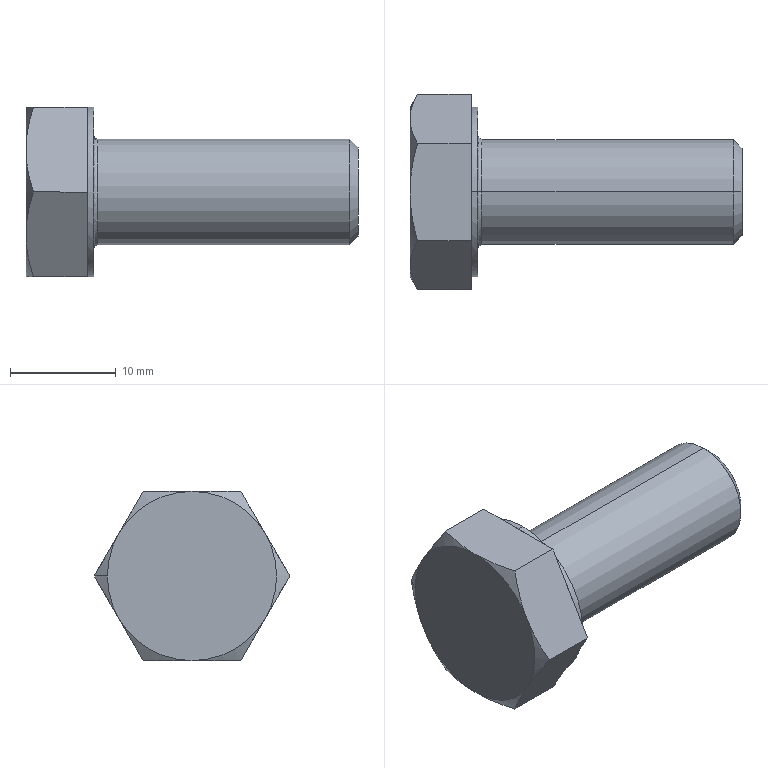Part | STEP file | Microwave Drying Flat Conveyor-hex screw gradeab_din_DIN EN 24017 - M10 x 25-N_Default | 1 solid | 30 faces | box 31.4 x 18.475 x 16 mm | volume 3356 mm3 | plane 15 | cone 9 | cylinder 4 | spline 2 | commonest cylinder face diameters 10 x2 16 x2
STEP:
#1=CARTESIAN_POINT('',(6.4,0.,5.4));
#2=VERTEX_POINT('',#1);
#3=CARTESIAN_POINT('',(6.4,0.,-5.4));
#4=VERTEX_POINT('',#3);
#5=CARTESIAN_POINT('',(6.4,0.,5.4));
#6=CARTESIAN_POINT('',(6.4,0.1651,5.4));
#7=CARTESIAN_POINT('',(6.4,0.4117,5.389));
#8=CARTESIAN_POINT('',(6.4,0.6977,5.356));
#9=CARTESIAN_POINT('',(6.4,0.8403,5.334));
#10=CARTESIAN_POINT('',(6.4,0.9013,5.324));
#11=CARTESIAN_POINT('',(6.4,0.942,5.317));
#12=CARTESIAN_POINT('',(6.4,0.9611,5.314));
#13=CARTESIAN_POINT('',(6.4,1.155,5.278));
#14=CARTESIAN_POINT('',(6.4,1.409,5.218));
#15=CARTESIAN_POINT('',(6.4,1.7,5.127));
#16=CARTESIAN_POINT('',(6.4,1.824,5.083));
#17=CARTESIAN_POINT('',(6.4,1.906,5.053));
#18=CARTESIAN_POINT('',(6.4,1.945,5.038));
#19=CARTESIAN_POINT('',(6.4,2.157,4.954));
#20=CARTESIAN_POINT('',(6.4,2.405,4.841));
#21=CARTESIAN_POINT('',(6.4,2.644,4.709));
#22=CARTESIAN_POINT('',(6.4,2.801,4.618));
#23=CARTESIAN_POINT('',(6.4,2.877,4.571));
#24=CARTESIAN_POINT('',(6.4,3.267,4.316));
#25=CARTESIAN_POINT('',(6.4,3.555,4.082));
#26=CARTESIAN_POINT('',(6.4,3.95,3.687));
#27=CARTESIAN_POINT('',(6.4,4.137,3.48));
#28=CARTESIAN_POINT('',(6.4,4.306,3.26));
#29=CARTESIAN_POINT('',(6.4,4.416,3.11));
#30=CARTESIAN_POINT('',(6.4,4.47,3.031));
#31=CARTESIAN_POINT('',(6.4,4.62,2.802));
#32=CARTESIAN_POINT('',(6.4,4.757,2.567));
#33=CARTESIAN_POINT('',(6.4,4.896,2.281));
#34=CARTESIAN_POINT('',(6.4,4.951,2.156));
#35=CARTESIAN_POINT('',(6.4,4.987,2.072));
#36=CARTESIAN_POINT('',(6.4,5.005,2.028));
#37=CARTESIAN_POINT('',(6.4,5.085,1.825));
#38=CARTESIAN_POINT('',(6.4,5.17,1.577));
#39=CARTESIAN_POINT('',(6.4,5.247,1.282));
#40=CARTESIAN_POINT('',(6.4,5.28,1.133));
#41=CARTESIAN_POINT('',(6.4,5.293,1.069));
#42=CARTESIAN_POINT('',(6.4,5.302,1.026));
#43=CARTESIAN_POINT('',(6.4,5.306,1.003));
#44=CARTESIAN_POINT('',(6.4,5.37,0.6582));
#45=CARTESIAN_POINT('',(6.4,5.4,0.3299));
#46=CARTESIAN_POINT('',(6.4,5.4,-0.165));
#47=CARTESIAN_POINT('',(6.4,5.389,-0.4115));
#48=CARTESIAN_POINT('',(6.4,5.356,-0.6976));
#49=CARTESIAN_POINT('',(6.4,5.335,-0.8402));
#50=CARTESIAN_POINT('',(6.4,5.324,-0.9013));
#51=CARTESIAN_POINT('',(6.4,5.317,-0.9419));
#52=CARTESIAN_POINT('',(6.4,5.314,-0.9611));
#53=CARTESIAN_POINT('',(6.4,5.278,-1.155));
#54=CARTESIAN_POINT('',(6.4,5.218,-1.409));
#55=CARTESIAN_POINT('',(6.4,5.127,-1.7));
#56=CARTESIAN_POINT('',(6.4,5.083,-1.824));
#57=CARTESIAN_POINT('',(6.4,5.053,-1.906));
#58=CARTESIAN_POINT('',(6.4,5.038,-1.945));
#59=CARTESIAN_POINT('',(6.4,4.954,-2.157));
#60=CARTESIAN_POINT('',(6.4,4.841,-2.405));
#61=CARTESIAN_POINT('',(6.4,4.709,-2.644));
#62=CARTESIAN_POINT('',(6.4,4.618,-2.801));
#63=CARTESIAN_POINT('',(6.4,4.571,-2.877));
#64=CARTESIAN_POINT('',(6.4,4.316,-3.267));
#65=CARTESIAN_POINT('',(6.4,4.082,-3.555));
#66=CARTESIAN_POINT('',(6.4,3.687,-3.95));
#67=CARTESIAN_POINT('',(6.4,3.48,-4.137));
#68=CARTESIAN_POINT('',(6.4,3.26,-4.306));
#69=CARTESIAN_POINT('',(6.4,3.11,-4.416));
#70=CARTESIAN_POINT('',(6.4,3.031,-4.47));
#71=CARTESIAN_POINT('',(6.4,2.802,-4.62));
#72=CARTESIAN_POINT('',(6.4,2.567,-4.757));
#73=CARTESIAN_POINT('',(6.4,2.281,-4.896));
#74=CARTESIAN_POINT('',(6.4,2.156,-4.951));
#75=CARTESIAN_POINT('',(6.4,2.072,-4.987));
#76=CARTESIAN_POINT('',(6.4,2.028,-5.005));
#77=CARTESIAN_POINT('',(6.4,1.825,-5.085));
#78=CARTESIAN_POINT('',(6.4,1.577,-5.17));
#79=CARTESIAN_POINT('',(6.4,1.282,-5.247));
#80=CARTESIAN_POINT('',(6.4,1.133,-5.28));
#81=CARTESIAN_POINT('',(6.4,1.069,-5.293));
#82=CARTESIAN_POINT('',(6.4,1.026,-5.302));
#83=CARTESIAN_POINT('',(6.4,1.003,-5.306));
#84=CARTESIAN_POINT('',(6.4,0.658,-5.37));
#85=CARTESIAN_POINT('',(6.4,0.3305,-5.4));
#86=CARTESIAN_POINT('',(6.4,0.,-5.4));
#87=B_SPLINE_CURVE_WITH_KNOTS('',3,(#5,#6,#7,#8,#9,#10,#11,#12,#13,#14,#15,#16,#17,#18,#19,#20,#21,#22,#23,#24,#25,#26,#27,#28,#29,#30,#31,#32,#33,#34,#35,#36,#37,#38,#39,#40,#41,#42,#43,#44,#45,#46,#47,#48,#49,#50,#51,#52,#53,#54,#55,#56,#57,#58,#59,#60,#61,#62,#63,#64,#65,#66,#67,#68,#69,#70,#71,#72,#73,#74,#75,#76,#77,#78,#79,#80,#81,#82,#83,#84,#85,#86),.UNSPECIFIED.,.F.,.F.,(4,1,1,1,2,2,1,1,2,2,1,2,2,2,1,2,2,1,1,2,2,1,1,1,2,2,2,1,1,1,2,2,1,1,2,2,1,2,2,2,1,2,2,1,1,2,2,1,1,1,2,2,4),(0.,0.03125,0.04687,0.05469,0.05859,0.0625,0.09375,0.1094,0.1172,0.125,0.1562,0.1719,0.1875,0.25,0.2812,0.2969,0.3125,0.3437,0.3594,0.3672,0.375,0.4062,0.4219,0.4297,0.4336,0.4375,0.5,0.5312,0.5469,0.5547,0.5586,0.5625,0.5937,0.6094,0.6172,0.625,0.6562,0.6719,0.6875,0.75,0.7812,0.7969,0.8125,0.8437,0.8594,0.8672,0.875,0.9062,0.9219,0.9297,0.9336,0.9375,1.),.UNSPECIFIED.);
#88=EDGE_CURVE('',#2,#4,#87,.T.);
#89=ORIENTED_EDGE('',*,*,#88,.F.);
#90=CARTESIAN_POINT('',(6.8,0.,5.));
#91=VERTEX_POINT('',#90);
#92=CARTESIAN_POINT('',(6.8,0.,5.4));
#93=DIRECTION('',(0.,-1.,0.));
#94=DIRECTION('',(0.,0.,1.));
#95=AXIS2_PLACEMENT_3D('',#92,#93,#94);
#96=CIRCLE('',#95,0.4);
#97=EDGE_CURVE('',#2,#91,#96,.T.);
#98=ORIENTED_EDGE('',*,*,#97,.T.);
#99=CARTESIAN_POINT('',(6.8,0.,-5.));
#100=VERTEX_POINT('',#99);
#101=CARTESIAN_POINT('',(6.8,0.,0.));
#102=DIRECTION('',(1.,0.,0.));
#103=DIRECTION('',(0.,0.,1.));
#104=AXIS2_PLACEMENT_3D('',#101,#102,#103);
#105=CIRCLE('',#104,5.);
#106=EDGE_CURVE('',#100,#91,#105,.T.);
#107=ORIENTED_EDGE('',*,*,#106,.F.);
#108=CARTESIAN_POINT('',(6.8,0.,-5.4));
#109=DIRECTION('',(0.,1.,0.));
#110=DIRECTION('',(0.,0.,-1.));
#111=AXIS2_PLACEMENT_3D('',#108,#109,#110);
#112=CIRCLE('',#111,0.4);
#113=EDGE_CURVE('',#4,#100,#112,.T.);
#114=ORIENTED_EDGE('',*,*,#113,.F.);
#115=EDGE_LOOP('',(#89,#98,#107,#114));
#116=FACE_OUTER_BOUND('',#115,.T.);
#117=CARTESIAN_POINT('',(6.4,0.,-5.4));
#118=CARTESIAN_POINT('',(6.4,10.8,-5.4));
#119=CARTESIAN_POINT('',(6.4,10.8,5.4));
#120=CARTESIAN_POINT('',(6.4,0.,5.4));
#121=CARTESIAN_POINT('',(6.4,0.,-5.166));
#122=CARTESIAN_POINT('',(6.4,10.331,-5.166));
#123=CARTESIAN_POINT('',(6.4,10.331,5.166));
#124=CARTESIAN_POINT('',(6.4,0.,5.166));
#125=CARTESIAN_POINT('',(6.566,0.,-5.));
#126=CARTESIAN_POINT('',(6.566,10.,-5.));
#127=CARTESIAN_POINT('',(6.566,10.,5.));
#128=CARTESIAN_POINT('',(6.566,0.,5.));
#129=CARTESIAN_POINT('',(6.8,0.,-5.));
#130=CARTESIAN_POINT('',(6.8,10.,-5.));
#131=CARTESIAN_POINT('',(6.8,10.,5.));
#132=CARTESIAN_POINT('',(6.8,0.,5.));
#133=(BOUNDED_SURFACE()B_SPLINE_SURFACE(3,3,((#117,#118,#119,#120),(#121,#122,#123,#124),(#125,#126,#127,#128),(#129,#130,#131,#132)),.UNSPECIFIED.,.F.,.F.,.F.)B_SPLINE_SURFACE_WITH_KNOTS((4,4),(4,4),(0.,1.),(0.,1.),.UNSPECIFIED.)GEOMETRIC_REPRESENTATION_ITEM()RATIONAL_B_SPLINE_SURFACE(((1.,0.3333,0.3333,1.),(0.8047,0.2682,0.2682,0.8047),(0.8047,0.2682,0.2682,0.8047),(1.,0.3333,0.3333,1.)))REPRESENTATION_ITEM('')SURFACE());
#134=ADVANCED_FACE('',(#116),#133,.F.);
#135=CARTESIAN_POINT('',(30.572,0.,5.));
#136=VERTEX_POINT('',#135);
#137=CARTESIAN_POINT('',(30.572,0.,-5.));
#138=VERTEX_POINT('',#137);
#139=CARTESIAN_POINT('',(30.572,0.,0.));
#140=DIRECTION('',(-1.,0.,0.));
#141=DIRECTION('',(0.,0.,1.));
#142=AXIS2_PLACEMENT_3D('',#139,#140,#141);
#143=CIRCLE('',#142,5.);
#144=EDGE_CURVE('',#136,#138,#143,.T.);
#145=ORIENTED_EDGE('',*,*,#144,.T.);
#146=CARTESIAN_POINT('',(0.,0.,-5.));
#147=DIRECTION('',(-1.,0.,0.));
#148=VECTOR('',#147,1000.);
#149=LINE('',#146,#148);
#150=EDGE_CURVE('',#138,#100,#149,.T.);
#151=ORIENTED_EDGE('',*,*,#150,.T.);
#152=ORIENTED_EDGE('',*,*,#106,.T.);
#153=CARTESIAN_POINT('',(0.,0.,5.));
#154=DIRECTION('',(-1.,0.,0.));
#155=VECTOR('',#154,1000.);
#156=LINE('',#153,#155);
#157=EDGE_CURVE('',#136,#91,#156,.T.);
#158=ORIENTED_EDGE('',*,*,#157,.F.);
#159=EDGE_LOOP('',(#145,#151,#152,#158));
#160=FACE_OUTER_BOUND('',#159,.T.);
#161=CARTESIAN_POINT('',(0.,0.,0.));
#162=DIRECTION('',(-1.,0.,0.));
#163=DIRECTION('',(0.,0.,1.));
#164=AXIS2_PLACEMENT_3D('',#161,#162,#163);
#165=CYLINDRICAL_SURFACE('',#164,5.);
#166=ADVANCED_FACE('',(#160),#165,.T.);
#167=CARTESIAN_POINT('',(31.4,0.,4.172));
#168=VERTEX_POINT('',#167);
#169=CARTESIAN_POINT('',(31.4,0.,-4.172));
#170=VERTEX_POINT('',#169);
#171=CARTESIAN_POINT('',(31.4,0.,0.));
#172=DIRECTION('',(-1.,0.,0.));
#173=DIRECTION('',(0.,0.,1.));
#174=AXIS2_PLACEMENT_3D('',#171,#172,#173);
#175=CIRCLE('',#174,4.172);
#176=EDGE_CURVE('',#168,#170,#175,.T.);
#177=ORIENTED_EDGE('',*,*,#176,.T.);
#178=CARTESIAN_POINT('',(30.572,0.,-5.));
#179=DIRECTION('',(-0.7071,0.,-0.7071));
#180=VECTOR('',#179,1000.);
#181=LINE('',#178,#180);
#182=EDGE_CURVE('',#170,#138,#181,.T.);
#183=ORIENTED_EDGE('',*,*,#182,.T.);
#184=ORIENTED_EDGE('',*,*,#144,.F.);
#185=CARTESIAN_POINT('',(30.572,0.,5.));
#186=DIRECTION('',(-0.7071,0.,0.7071));
#187=VECTOR('',#186,1000.);
#188=LINE('',#185,#187);
#189=EDGE_CURVE('',#168,#136,#188,.T.);
#190=ORIENTED_EDGE('',*,*,#189,.F.);
#191=EDGE_LOOP('',(#177,#183,#184,#190));
#192=FACE_OUTER_BOUND('',#191,.T.);
#193=CARTESIAN_POINT('',(30.572,0.,0.));
#194=DIRECTION('',(-1.,0.,0.));
#195=DIRECTION('',(0.,0.,1.));
#196=AXIS2_PLACEMENT_3D('',#193,#194,#195);
#197=CONICAL_SURFACE('',#196,5.,0.7854);
#198=ADVANCED_FACE('',(#192),#197,.T.);
#199=CARTESIAN_POINT('',(6.4,0.,-8.));
#200=VERTEX_POINT('',#199);
#201=CARTESIAN_POINT('',(6.4,0.,8.));
#202=VERTEX_POINT('',#201);
#203=CARTESIAN_POINT('',(6.4,0.,0.));
#204=DIRECTION('',(1.,0.,0.));
#205=DIRECTION('',(0.,0.,1.));
#206=AXIS2_PLACEMENT_3D('',#203,#204,#205);
#207=CIRCLE('',#206,8.);
#208=EDGE_CURVE('',#200,#202,#207,.T.);
#209=ORIENTED_EDGE('',*,*,#208,.F.);
#210=CARTESIAN_POINT('',(5.8,0.,-8.));
#211=VERTEX_POINT('',#210);
#212=CARTESIAN_POINT('',(0.,0.,-8.));
#213=DIRECTION('',(-1.,0.,0.));
#214=VECTOR('',#213,1000.);
#215=LINE('',#212,#214);
#216=EDGE_CURVE('',#200,#211,#215,.T.);
#217=ORIENTED_EDGE('',*,*,#216,.T.);
#218=CARTESIAN_POINT('',(5.8,6.928,-4.));
#219=VERTEX_POINT('',#218);
#220=CARTESIAN_POINT('',(5.8,0.,0.));
#221=DIRECTION('',(1.,0.,0.));
#222=DIRECTION('',(0.,0.,1.));
#223=AXIS2_PLACEMENT_3D('',#220,#221,#222);
#224=CIRCLE('',#223,8.);
#225=EDGE_CURVE('',#211,#219,#224,.T.);
#226=ORIENTED_EDGE('',*,*,#225,.T.);
#227=CARTESIAN_POINT('',(5.8,6.928,4.));
#228=VERTEX_POINT('',#227);
#229=CARTESIAN_POINT('',(5.8,0.,0.));
#230=DIRECTION('',(1.,0.,0.));
#231=DIRECTION('',(0.,0.,1.));
#232=AXIS2_PLACEMENT_3D('',#229,#230,#231);
#233=CIRCLE('',#232,8.);
#234=EDGE_CURVE('',#219,#228,#233,.T.);
#235=ORIENTED_EDGE('',*,*,#234,.T.);
#236=CARTESIAN_POINT('',(5.8,0.,8.));
#237=VERTEX_POINT('',#236);
#238=CARTESIAN_POINT('',(5.8,0.,0.));
#239=DIRECTION('',(1.,0.,0.));
#240=DIRECTION('',(0.,0.,1.));
#241=AXIS2_PLACEMENT_3D('',#238,#239,#240);
#242=CIRCLE('',#241,8.);
#243=EDGE_CURVE('',#228,#237,#242,.T.);
#244=ORIENTED_EDGE('',*,*,#243,.T.);
#245=CARTESIAN_POINT('',(0.,0.,8.));
#246=DIRECTION('',(-1.,0.,0.));
#247=VECTOR('',#246,1000.);
#248=LINE('',#245,#247);
#249=EDGE_CURVE('',#202,#237,#248,.T.);
#250=ORIENTED_EDGE('',*,*,#249,.F.);
#251=EDGE_LOOP('',(#209,#217,#226,#235,#244,#250));
#252=FACE_OUTER_BOUND('',#251,.T.);
#253=CARTESIAN_POINT('',(0.,0.,0.));
#254=DIRECTION('',(-1.,0.,0.));
#255=DIRECTION('',(0.,0.,1.));
#256=AXIS2_PLACEMENT_3D('',#253,#254,#255);
#257=CYLINDRICAL_SURFACE('',#256,8.);
#258=ADVANCED_FACE('',(#252),#257,.T.);
#259=CARTESIAN_POINT('',(0.,6.928,-4.));
#260=VERTEX_POINT('',#259);
#261=CARTESIAN_POINT('',(0.,8.,0.));
#262=VERTEX_POINT('',#261);
#263=CARTESIAN_POINT('',(0.,0.,0.));
#264=DIRECTION('',(1.,0.,0.));
#265=DIRECTION('',(0.,1.,0.));
#266=AXIS2_PLACEMENT_3D('',#263,#264,#265);
#267=CIRCLE('',#266,8.);
#268=EDGE_CURVE('',#260,#262,#267,.T.);
#269=ORIENTED_EDGE('',*,*,#268,.T.);
#270=CARTESIAN_POINT('',(0.7145,9.238,0.));
#271=VERTEX_POINT('',#270);
#272=CARTESIAN_POINT('',(0.7188,9.245,0.));
#273=DIRECTION('',(0.5,0.866,0.));
#274=VECTOR('',#273,1000.);
#275=LINE('',#272,#274);
#276=EDGE_CURVE('',#262,#271,#275,.T.);
#277=ORIENTED_EDGE('',*,*,#276,.T.);
#278=CARTESIAN_POINT('',(0.7145,9.238,0.));
#279=CARTESIAN_POINT('',(0.4967,8.86,-0.6534));
#280=CARTESIAN_POINT('',(0.3171,8.48,-1.312));
#281=CARTESIAN_POINT('',(0.06831,7.711,-2.644));
#282=CARTESIAN_POINT('',(0.,7.322,-3.317));
#283=CARTESIAN_POINT('',(0.,6.928,-4.));
#284=B_SPLINE_CURVE_WITH_KNOTS('',3,(#278,#279,#280,#281,#282,#283),.UNSPECIFIED.,.F.,.F.,(4,2,4),(0.,0.002337,0.004674),.UNSPECIFIED.);
#285=EDGE_CURVE('',#271,#260,#284,.T.);
#286=ORIENTED_EDGE('',*,*,#285,.T.);
#287=EDGE_LOOP('',(#269,#277,#286));
#288=FACE_OUTER_BOUND('',#287,.T.);
#289=CARTESIAN_POINT('',(0.7188,0.,0.));
#290=DIRECTION('',(1.,0.,0.));
#291=DIRECTION('',(0.,1.,0.));
#292=AXIS2_PLACEMENT_3D('',#289,#290,#291);
#293=CONICAL_SURFACE('',#292,9.245,1.047);
#294=ADVANCED_FACE('',(#288),#293,.T.);
#295=ORIENTED_EDGE('',*,*,#150,.F.);
#296=CARTESIAN_POINT('',(30.572,0.,0.));
#297=DIRECTION('',(-1.,0.,0.));
#298=DIRECTION('',(0.,0.,1.));
#299=AXIS2_PLACEMENT_3D('',#296,#297,#298);
#300=CIRCLE('',#299,5.);
#301=EDGE_CURVE('',#138,#136,#300,.T.);
#302=ORIENTED_EDGE('',*,*,#301,.T.);
#303=ORIENTED_EDGE('',*,*,#157,.T.);
#304=CARTESIAN_POINT('',(6.8,0.,0.));
#305=DIRECTION('',(1.,0.,0.));
#306=DIRECTION('',(0.,0.,1.));
#307=AXIS2_PLACEMENT_3D('',#304,#305,#306);
#308=CIRCLE('',#307,5.);
#309=EDGE_CURVE('',#91,#100,#308,.T.);
#310=ORIENTED_EDGE('',*,*,#309,.T.);
#311=EDGE_LOOP('',(#295,#302,#303,#310));
#312=FACE_OUTER_BOUND('',#311,.T.);
#313=CARTESIAN_POINT('',(0.,0.,0.));
#314=DIRECTION('',(-1.,0.,0.));
#315=DIRECTION('',(0.,0.,1.));
#316=AXIS2_PLACEMENT_3D('',#313,#314,#315);
#317=CYLINDRICAL_SURFACE('',#316,5.);
#318=ADVANCED_FACE('',(#312),#317,.T.);
#319=ORIENTED_EDGE('',*,*,#97,.F.);
#320=CARTESIAN_POINT('',(6.4,0.,-5.4));
#321=CARTESIAN_POINT('',(6.4,-0.1651,-5.4));
#322=CARTESIAN_POINT('',(6.4,-0.4117,-5.389));
#323=CARTESIAN_POINT('',(6.4,-0.6977,-5.356));
#324=CARTESIAN_POINT('',(6.4,-0.8403,-5.334));
#325=CARTESIAN_POINT('',(6.4,-0.9013,-5.324));
#326=CARTESIAN_POINT('',(6.4,-0.942,-5.317));
#327=CARTESIAN_POINT('',(6.4,-0.9611,-5.314));
#328=CARTESIAN_POINT('',(6.4,-1.155,-5.278));
#329=CARTESIAN_POINT('',(6.4,-1.409,-5.218));
#330=CARTESIAN_POINT('',(6.4,-1.7,-5.127));
#331=CARTESIAN_POINT('',(6.4,-1.824,-5.083));
#332=CARTESIAN_POINT('',(6.4,-1.906,-5.053));
#333=CARTESIAN_POINT('',(6.4,-1.945,-5.038));
#334=CARTESIAN_POINT('',(6.4,-2.157,-4.954));
#335=CARTESIAN_POINT('',(6.4,-2.405,-4.841));
#336=CARTESIAN_POINT('',(6.4,-2.644,-4.709));
#337=CARTESIAN_POINT('',(6.4,-2.801,-4.618));
#338=CARTESIAN_POINT('',(6.4,-2.877,-4.571));
#339=CARTESIAN_POINT('',(6.4,-3.267,-4.316));
#340=CARTESIAN_POINT('',(6.4,-3.555,-4.082));
#341=CARTESIAN_POINT('',(6.4,-3.95,-3.687));
#342=CARTESIAN_POINT('',(6.4,-4.137,-3.48));
#343=CARTESIAN_POINT('',(6.4,-4.306,-3.26));
#344=CARTESIAN_POINT('',(6.4,-4.416,-3.11));
#345=CARTESIAN_POINT('',(6.4,-4.47,-3.031));
#346=CARTESIAN_POINT('',(6.4,-4.62,-2.802));
#347=CARTESIAN_POINT('',(6.4,-4.757,-2.567));
#348=CARTESIAN_POINT('',(6.4,-4.896,-2.281));
#349=CARTESIAN_POINT('',(6.4,-4.951,-2.156));
#350=CARTESIAN_POINT('',(6.4,-4.987,-2.072));
#351=CARTESIAN_POINT('',(6.4,-5.005,-2.028));
#352=CARTESIAN_POINT('',(6.4,-5.085,-1.825));
#353=CARTESIAN_POINT('',(6.4,-5.17,-1.577));
#354=CARTESIAN_POINT('',(6.4,-5.247,-1.282));
#355=CARTESIAN_POINT('',(6.4,-5.28,-1.133));
#356=CARTESIAN_POINT('',(6.4,-5.293,-1.069));
#357=CARTESIAN_POINT('',(6.4,-5.302,-1.026));
#358=CARTESIAN_POINT('',(6.4,-5.306,-1.003));
#359=CARTESIAN_POINT('',(6.4,-5.37,-0.6582));
#360=CARTESIAN_POINT('',(6.4,-5.4,-0.3299));
#361=CARTESIAN_POINT('',(6.4,-5.4,0.165));
#362=CARTESIAN_POINT('',(6.4,-5.389,0.4115));
#363=CARTESIAN_POINT('',(6.4,-5.356,0.6976));
#364=CARTESIAN_POINT('',(6.4,-5.335,0.8402));
#365=CARTESIAN_POINT('',(6.4,-5.324,0.9013));
#366=CARTESIAN_POINT('',(6.4,-5.317,0.9419));
#367=CARTESIAN_POINT('',(6.4,-5.314,0.9611));
#368=CARTESIAN_POINT('',(6.4,-5.278,1.155));
#369=CARTESIAN_POINT('',(6.4,-5.218,1.409));
#370=CARTESIAN_POINT('',(6.4,-5.127,1.7));
#371=CARTESIAN_POINT('',(6.4,-5.083,1.824));
#372=CARTESIAN_POINT('',(6.4,-5.053,1.906));
#373=CARTESIAN_POINT('',(6.4,-5.038,1.945));
#374=CARTESIAN_POINT('',(6.4,-4.954,2.157));
#375=CARTESIAN_POINT('',(6.4,-4.841,2.405));
#376=CARTESIAN_POINT('',(6.4,-4.709,2.644));
#377=CARTESIAN_POINT('',(6.4,-4.618,2.801));
#378=CARTESIAN_POINT('',(6.4,-4.571,2.877));
#379=CARTESIAN_POINT('',(6.4,-4.316,3.267));
#380=CARTESIAN_POINT('',(6.4,-4.082,3.555));
#381=CARTESIAN_POINT('',(6.4,-3.687,3.95));
#382=CARTESIAN_POINT('',(6.4,-3.48,4.137));
#383=CARTESIAN_POINT('',(6.4,-3.26,4.306));
#384=CARTESIAN_POINT('',(6.4,-3.11,4.416));
#385=CARTESIAN_POINT('',(6.4,-3.031,4.47));
#386=CARTESIAN_POINT('',(6.4,-2.802,4.62));
#387=CARTESIAN_POINT('',(6.4,-2.567,4.757));
#388=CARTESIAN_POINT('',(6.4,-2.281,4.896));
#389=CARTESIAN_POINT('',(6.4,-2.156,4.951));
#390=CARTESIAN_POINT('',(6.4,-2.072,4.987));
#391=CARTESIAN_POINT('',(6.4,-2.028,5.005));
#392=CARTESIAN_POINT('',(6.4,-1.825,5.085));
#393=CARTESIAN_POINT('',(6.4,-1.577,5.17));
#394=CARTESIAN_POINT('',(6.4,-1.282,5.247));
#395=CARTESIAN_POINT('',(6.4,-1.133,5.28));
#396=CARTESIAN_POINT('',(6.4,-1.069,5.293));
#397=CARTESIAN_POINT('',(6.4,-1.026,5.302));
#398=CARTESIAN_POINT('',(6.4,-1.003,5.306));
#399=CARTESIAN_POINT('',(6.4,-0.658,5.37));
#400=CARTESIAN_POINT('',(6.4,-0.3305,5.4));
#401=CARTESIAN_POINT('',(6.4,0.,5.4));
#402=B_SPLINE_CURVE_WITH_KNOTS('',3,(#320,#321,#322,#323,#324,#325,#326,#327,#328,#329,#330,#331,#332,#333,#334,#335,#336,#337,#338,#339,#340,#341,#342,#343,#344,#345,#346,#347,#348,#349,#350,#351,#352,#353,#354,#355,#356,#357,#358,#359,#360,#361,#362,#363,#364,#365,#366,#367,#368,#369,#370,#371,#372,#373,#374,#375,#376,#377,#378,#379,#380,#381,#382,#383,#384,#385,#386,#387,#388,#389,#390,#391,#392,#393,#394,#395,#396,#397,#398,#399,#400,#401),.UNSPECIFIED.,.F.,.F.,(4,1,1,1,2,2,1,1,2,2,1,2,2,2,1,2,2,1,1,2,2,1,1,1,2,2,2,1,1,1,2,2,1,1,2,2,1,2,2,2,1,2,2,1,1,2,2,1,1,1,2,2,4),(0.,0.03125,0.04687,0.05469,0.05859,0.0625,0.09375,0.1094,0.1172,0.125,0.1563,0.1719,0.1875,0.25,0.2813,0.2969,0.3125,0.3438,0.3594,0.3672,0.375,0.4063,0.4219,0.4297,0.4336,0.4375,0.5,0.5313,0.5469,0.5547,0.5586,0.5625,0.5938,0.6094,0.6172,0.625,0.6563,0.6719,0.6875,0.75,0.7813,0.7969,0.8125,0.8438,0.8594,0.8672,0.875,0.9063,0.9219,0.9297,0.9336,0.9375,1.),.UNSPECIFIED.);
#403=EDGE_CURVE('',#4,#2,#402,.T.);
#404=ORIENTED_EDGE('',*,*,#403,.F.);
#405=ORIENTED_EDGE('',*,*,#113,.T.);
#406=ORIENTED_EDGE('',*,*,#309,.F.);
#407=EDGE_LOOP('',(#319,#404,#405,#406));
#408=FACE_OUTER_BOUND('',#407,.T.);
#409=CARTESIAN_POINT('',(6.4,0.,5.4));
#410=CARTESIAN_POINT('',(6.4,-10.8,5.4));
#411=CARTESIAN_POINT('',(6.4,-10.8,-5.4));
#412=CARTESIAN_POINT('',(6.4,0.,-5.4));
#413=CARTESIAN_POINT('',(6.4,0.,5.166));
#414=CARTESIAN_POINT('',(6.4,-10.331,5.166));
#415=CARTESIAN_POINT('',(6.4,-10.331,-5.166));
#416=CARTESIAN_POINT('',(6.4,0.,-5.166));
#417=CARTESIAN_POINT('',(6.566,0.,5.));
#418=CARTESIAN_POINT('',(6.566,-10.,5.));
#419=CARTESIAN_POINT('',(6.566,-10.,-5.));
#420=CARTESIAN_POINT('',(6.566,0.,-5.));
#421=CARTESIAN_POINT('',(6.8,0.,5.));
#422=CARTESIAN_POINT('',(6.8,-10.,5.));
#423=CARTESIAN_POINT('',(6.8,-10.,-5.));
#424=CARTESIAN_POINT('',(6.8,0.,-5.));
#425=(BOUNDED_SURFACE()B_SPLINE_SURFACE(3,3,((#409,#410,#411,#412),(#413,#414,#415,#416),(#417,#418,#419,#420),(#421,#422,#423,#424)),.UNSPECIFIED.,.F.,.F.,.F.)B_SPLINE_SURFACE_WITH_KNOTS((4,4),(4,4),(0.,1.),(0.,1.),.UNSPECIFIED.)GEOMETRIC_REPRESENTATION_ITEM()RATIONAL_B_SPLINE_SURFACE(((1.,0.3333,0.3333,1.),(0.8047,0.2682,0.2682,0.8047),(0.8047,0.2682,0.2682,0.8047),(1.,0.3333,0.3333,1.)))REPRESENTATION_ITEM('')SURFACE());
#426=ADVANCED_FACE('',(#408),#425,.F.);
#427=ORIENTED_EDGE('',*,*,#182,.F.);
#428=CARTESIAN_POINT('',(31.4,0.,0.));
#429=DIRECTION('',(-1.,0.,0.));
#430=DIRECTION('',(0.,0.,1.));
#431=AXIS2_PLACEMENT_3D('',#428,#429,#430);
#432=CIRCLE('',#431,4.172);
#433=EDGE_CURVE('',#170,#168,#432,.T.);
#434=ORIENTED_EDGE('',*,*,#433,.T.);
#435=ORIENTED_EDGE('',*,*,#189,.T.);
#436=ORIENTED_EDGE('',*,*,#301,.F.);
#437=EDGE_LOOP('',(#427,#434,#435,#436));
#438=FACE_OUTER_BOUND('',#437,.T.);
#439=CARTESIAN_POINT('',(30.572,0.,0.));
#440=DIRECTION('',(-1.,0.,0.));
#441=DIRECTION('',(0.,0.,1.));
#442=AXIS2_PLACEMENT_3D('',#439,#440,#441);
#443=CONICAL_SURFACE('',#442,5.,0.7854);
#444=ADVANCED_FACE('',(#438),#443,.T.);
#445=CARTESIAN_POINT('',(6.4,0.,0.));
#446=DIRECTION('',(1.,0.,0.));
#447=DIRECTION('',(0.,0.,1.));
#448=AXIS2_PLACEMENT_3D('',#445,#446,#447);
#449=CIRCLE('',#448,8.);
#450=EDGE_CURVE('',#202,#200,#449,.T.);
#451=ORIENTED_EDGE('',*,*,#450,.T.);
#452=ORIENTED_EDGE('',*,*,#208,.T.);
#453=EDGE_LOOP('',(#451,#452));
#454=FACE_OUTER_BOUND('',#453,.T.);
#455=ORIENTED_EDGE('',*,*,#403,.T.);
#456=ORIENTED_EDGE('',*,*,#88,.T.);
#457=EDGE_LOOP('',(#455,#456));
#458=FACE_BOUND('',#457,.T.);
#459=CARTESIAN_POINT('',(6.4,9.238,0.));
#460=DIRECTION('',(1.,0.,0.));
#461=DIRECTION('',(0.,0.,-1.));
#462=AXIS2_PLACEMENT_3D('',#459,#460,#461);
#463=PLANE('',#462);
#464=ADVANCED_FACE('',(#454,#458),#463,.T.);
#465=ORIENTED_EDGE('',*,*,#176,.F.);
#466=ORIENTED_EDGE('',*,*,#433,.F.);
#467=EDGE_LOOP('',(#465,#466));
#468=FACE_OUTER_BOUND('',#467,.T.);
#469=CARTESIAN_POINT('',(31.4,0.,0.));
#470=DIRECTION('',(-1.,0.,0.));
#471=DIRECTION('',(0.,0.,1.));
#472=AXIS2_PLACEMENT_3D('',#469,#470,#471);
#473=PLANE('',#472);
#474=ADVANCED_FACE('',(#468),#473,.F.);
#475=ORIENTED_EDGE('',*,*,#216,.F.);
#476=ORIENTED_EDGE('',*,*,#450,.F.);
#477=ORIENTED_EDGE('',*,*,#249,.T.);
#478=CARTESIAN_POINT('',(5.8,-6.928,4.));
#479=VERTEX_POINT('',#478);
#480=CARTESIAN_POINT('',(5.8,0.,0.));
#481=DIRECTION('',(1.,0.,0.));
#482=DIRECTION('',(0.,0.,1.));
#483=AXIS2_PLACEMENT_3D('',#480,#481,#482);
#484=CIRCLE('',#483,8.);
#485=EDGE_CURVE('',#237,#479,#484,.T.);
#486=ORIENTED_EDGE('',*,*,#485,.T.);
#487=CARTESIAN_POINT('',(5.8,-6.928,-4.));
#488=VERTEX_POINT('',#487);
#489=CARTESIAN_POINT('',(5.8,0.,0.));
#490=DIRECTION('',(1.,0.,0.));
#491=DIRECTION('',(0.,0.,1.));
#492=AXIS2_PLACEMENT_3D('',#489,#490,#491);
#493=CIRCLE('',#492,8.);
#494=EDGE_CURVE('',#479,#488,#493,.T.);
#495=ORIENTED_EDGE('',*,*,#494,.T.);
#496=CARTESIAN_POINT('',(5.8,0.,0.));
#497=DIRECTION('',(1.,0.,0.));
#498=DIRECTION('',(0.,0.,1.));
#499=AXIS2_PLACEMENT_3D('',#496,#497,#498);
#500=CIRCLE('',#499,8.);
#501=EDGE_CURVE('',#488,#211,#500,.T.);
#502=ORIENTED_EDGE('',*,*,#501,.T.);
#503=EDGE_LOOP('',(#475,#476,#477,#486,#495,#502));
#504=FACE_OUTER_BOUND('',#503,.T.);
#505=CARTESIAN_POINT('',(0.,0.,0.));
#506=DIRECTION('',(-1.,0.,0.));
#507=DIRECTION('',(0.,0.,1.));
#508=AXIS2_PLACEMENT_3D('',#505,#506,#507);
#509=CYLINDRICAL_SURFACE('',#508,8.);
#510=ADVANCED_FACE('',(#504),#509,.T.);
#511=CARTESIAN_POINT('',(5.8,4.619,8.));
#512=VERTEX_POINT('',#511);
#513=CARTESIAN_POINT('',(5.8,8.,8.));
#514=DIRECTION('',(0.,-1.,0.));
#515=VECTOR('',#514,1000.);
#516=LINE('',#513,#515);
#517=EDGE_CURVE('',#512,#237,#516,.T.);
#518=ORIENTED_EDGE('',*,*,#517,.T.);
#519=ORIENTED_EDGE('',*,*,#243,.F.);
#520=CARTESIAN_POINT('',(5.8,6.928,4.));
#521=DIRECTION('',(0.,-0.5,0.866));
#522=VECTOR('',#521,1000.);
#523=LINE('',#520,#522);
#524=EDGE_CURVE('',#228,#512,#523,.T.);
#525=ORIENTED_EDGE('',*,*,#524,.T.);
#526=EDGE_LOOP('',(#518,#519,#525));
#527=FACE_OUTER_BOUND('',#526,.T.);
#528=CARTESIAN_POINT('',(5.8,8.,0.));
#529=DIRECTION('',(1.,0.,0.));
#530=DIRECTION('',(0.,0.,-1.));
#531=AXIS2_PLACEMENT_3D('',#528,#529,#530);
#532=PLANE('',#531);
#533=ADVANCED_FACE('',(#527),#532,.T.);
#534=CARTESIAN_POINT('',(5.8,9.238,0.));
#535=VERTEX_POINT('',#534);
#536=CARTESIAN_POINT('',(5.8,9.238,0.));
#537=DIRECTION('',(0.,-0.5,0.866));
#538=VECTOR('',#537,1000.);
#539=LINE('',#536,#538);
#540=EDGE_CURVE('',#535,#228,#539,.T.);
#541=ORIENTED_EDGE('',*,*,#540,.T.);
#542=ORIENTED_EDGE('',*,*,#234,.F.);
#543=CARTESIAN_POINT('',(5.8,6.928,-4.));
#544=DIRECTION('',(0.,0.5,0.866));
#545=VECTOR('',#544,1000.);
#546=LINE('',#543,#545);
#547=EDGE_CURVE('',#219,#535,#546,.T.);
#548=ORIENTED_EDGE('',*,*,#547,.T.);
#549=EDGE_LOOP('',(#541,#542,#548));
#550=FACE_OUTER_BOUND('',#549,.T.);
#551=CARTESIAN_POINT('',(5.8,8.,0.));
#552=DIRECTION('',(1.,0.,0.));
#553=DIRECTION('',(0.,0.,-1.));
#554=AXIS2_PLACEMENT_3D('',#551,#552,#553);
#555=PLANE('',#554);
#556=ADVANCED_FACE('',(#550),#555,.T.);
#557=ORIENTED_EDGE('',*,*,#225,.F.);
#558=CARTESIAN_POINT('',(5.8,4.619,-8.));
#559=VERTEX_POINT('',#558);
#560=CARTESIAN_POINT('',(5.8,8.,-8.));
#561=DIRECTION('',(0.,1.,0.));
#562=VECTOR('',#561,1000.);
#563=LINE('',#560,#562);
#564=EDGE_CURVE('',#211,#559,#563,.T.);
#565=ORIENTED_EDGE('',*,*,#564,.T.);
#566=CARTESIAN_POINT('',(5.8,4.619,-8.));
#567=DIRECTION('',(0.,0.5,0.866));
#568=VECTOR('',#567,1000.);
#569=LINE('',#566,#568);
#570=EDGE_CURVE('',#559,#219,#569,.T.);
#571=ORIENTED_EDGE('',*,*,#570,.T.);
#572=EDGE_LOOP('',(#557,#565,#571));
#573=FACE_OUTER_BOUND('',#572,.T.);
#574=CARTESIAN_POINT('',(5.8,8.,0.));
#575=DIRECTION('',(1.,0.,0.));
#576=DIRECTION('',(0.,0.,-1.));
#577=AXIS2_PLACEMENT_3D('',#574,#575,#576);
#578=PLANE('',#577);
#579=ADVANCED_FACE('',(#573),#578,.T.);
#580=CARTESIAN_POINT('',(5.8,-4.619,-8.));
#581=VERTEX_POINT('',#580);
#582=CARTESIAN_POINT('',(5.8,8.,-8.));
#583=DIRECTION('',(0.,1.,0.));
#584=VECTOR('',#583,1000.);
#585=LINE('',#582,#584);
#586=EDGE_CURVE('',#581,#211,#585,.T.);
#587=ORIENTED_EDGE('',*,*,#586,.T.);
#588=ORIENTED_EDGE('',*,*,#501,.F.);
#589=CARTESIAN_POINT('',(5.8,-6.928,-4.));
#590=DIRECTION('',(0.,0.5,-0.866));
#591=VECTOR('',#590,1000.);
#592=LINE('',#589,#591);
#593=EDGE_CURVE('',#488,#581,#592,.T.);
#594=ORIENTED_EDGE('',*,*,#593,.T.);
#595=EDGE_LOOP('',(#587,#588,#594));
#596=FACE_OUTER_BOUND('',#595,.T.);
#597=CARTESIAN_POINT('',(5.8,8.,0.));
#598=DIRECTION('',(1.,0.,0.));
#599=DIRECTION('',(0.,0.,-1.));
#600=AXIS2_PLACEMENT_3D('',#597,#598,#599);
#601=PLANE('',#600);
#602=ADVANCED_FACE('',(#596),#601,.T.);
#603=CARTESIAN_POINT('',(5.8,-9.238,0.));
#604=VERTEX_POINT('',#603);
#605=CARTESIAN_POINT('',(5.8,-9.238,0.));
#606=DIRECTION('',(0.,0.5,-0.866));
#607=VECTOR('',#606,1000.);
#608=LINE('',#605,#607);
#609=EDGE_CURVE('',#604,#488,#608,.T.);
#610=ORIENTED_EDGE('',*,*,#609,.T.);
#611=ORIENTED_EDGE('',*,*,#494,.F.);
#612=CARTESIAN_POINT('',(5.8,-6.928,4.));
#613=DIRECTION('',(0.,-0.5,-0.866));
#614=VECTOR('',#613,1000.);
#615=LINE('',#612,#614);
#616=EDGE_CURVE('',#479,#604,#615,.T.);
#617=ORIENTED_EDGE('',*,*,#616,.T.);
#618=EDGE_LOOP('',(#610,#611,#617));
#619=FACE_OUTER_BOUND('',#618,.T.);
#620=CARTESIAN_POINT('',(5.8,8.,0.));
#621=DIRECTION('',(1.,0.,0.));
#622=DIRECTION('',(0.,0.,-1.));
#623=AXIS2_PLACEMENT_3D('',#620,#621,#622);
#624=PLANE('',#623);
#625=ADVANCED_FACE('',(#619),#624,.T.);
#626=CARTESIAN_POINT('',(5.8,-4.619,8.));
#627=VERTEX_POINT('',#626);
#628=CARTESIAN_POINT('',(5.8,-4.619,8.));
#629=DIRECTION('',(0.,-0.5,-0.866));
#630=VECTOR('',#629,1000.);
#631=LINE('',#628,#630);
#632=EDGE_CURVE('',#627,#479,#631,.T.);
#633=ORIENTED_EDGE('',*,*,#632,.T.);
#634=ORIENTED_EDGE('',*,*,#485,.F.);
#635=CARTESIAN_POINT('',(5.8,8.,8.));
#636=DIRECTION('',(0.,-1.,0.));
#637=VECTOR('',#636,1000.);
#638=LINE('',#635,#637);
#639=EDGE_CURVE('',#237,#627,#638,.T.);
#640=ORIENTED_EDGE('',*,*,#639,.T.);
#641=EDGE_LOOP('',(#633,#634,#640));
#642=FACE_OUTER_BOUND('',#641,.T.);
#643=CARTESIAN_POINT('',(5.8,8.,0.));
#644=DIRECTION('',(1.,0.,0.));
#645=DIRECTION('',(0.,0.,-1.));
#646=AXIS2_PLACEMENT_3D('',#643,#644,#645);
#647=PLANE('',#646);
#648=ADVANCED_FACE('',(#642),#647,.T.);
#649=CARTESIAN_POINT('',(0.7145,4.619,8.));
#650=VERTEX_POINT('',#649);
#651=CARTESIAN_POINT('',(6.4,4.619,8.));
#652=DIRECTION('',(1.,0.,0.));
#653=VECTOR('',#652,1000.);
#654=LINE('',#651,#653);
#655=EDGE_CURVE('',#650,#512,#654,.T.);
#656=ORIENTED_EDGE('',*,*,#655,.F.);
#657=CARTESIAN_POINT('',(0.,0.,8.));
#658=VERTEX_POINT('',#657);
#659=CARTESIAN_POINT('',(0.,0.,8.));
#660=CARTESIAN_POINT('',(0.,0.7882,8.));
#661=CARTESIAN_POINT('',(0.06831,1.566,8.));
#662=CARTESIAN_POINT('',(0.3171,3.104,8.));
#663=CARTESIAN_POINT('',(0.4967,3.864,8.));
#664=CARTESIAN_POINT('',(0.7145,4.619,8.));
#665=B_SPLINE_CURVE_WITH_KNOTS('',3,(#659,#660,#661,#662,#663,#664),.UNSPECIFIED.,.F.,.F.,(4,2,4),(0.,0.002337,0.004674),.UNSPECIFIED.);
#666=EDGE_CURVE('',#658,#650,#665,.T.);
#667=ORIENTED_EDGE('',*,*,#666,.F.);
#668=CARTESIAN_POINT('',(0.7145,-4.619,8.));
#669=VERTEX_POINT('',#668);
#670=CARTESIAN_POINT('',(0.7145,-4.619,8.));
#671=CARTESIAN_POINT('',(0.4967,-3.864,8.));
#672=CARTESIAN_POINT('',(0.3171,-3.104,8.));
#673=CARTESIAN_POINT('',(0.06831,-1.566,8.));
#674=CARTESIAN_POINT('',(0.,-0.7882,8.));
#675=CARTESIAN_POINT('',(0.,0.,8.));
#676=B_SPLINE_CURVE_WITH_KNOTS('',3,(#670,#671,#672,#673,#674,#675),.UNSPECIFIED.,.F.,.F.,(4,2,4),(0.,0.002337,0.004674),.UNSPECIFIED.);
#677=EDGE_CURVE('',#669,#658,#676,.T.);
#678=ORIENTED_EDGE('',*,*,#677,.F.);
#679=CARTESIAN_POINT('',(6.4,-4.619,8.));
#680=DIRECTION('',(-1.,0.,0.));
#681=VECTOR('',#680,1000.);
#682=LINE('',#679,#681);
#683=EDGE_CURVE('',#627,#669,#682,.T.);
#684=ORIENTED_EDGE('',*,*,#683,.F.);
#685=ORIENTED_EDGE('',*,*,#639,.F.);
#686=ORIENTED_EDGE('',*,*,#517,.F.);
#687=EDGE_LOOP('',(#656,#667,#678,#684,#685,#686));
#688=FACE_OUTER_BOUND('',#687,.T.);
#689=CARTESIAN_POINT('',(6.4,4.619,8.));
#690=DIRECTION('',(0.,0.,-1.));
#691=DIRECTION('',(0.,1.,0.));
#692=AXIS2_PLACEMENT_3D('',#689,#690,#691);
#693=PLANE('',#692);
#694=ADVANCED_FACE('',(#688),#693,.F.);
#695=CARTESIAN_POINT('',(6.4,9.238,0.));
#696=DIRECTION('',(1.,0.,0.));
#697=VECTOR('',#696,1000.);
#698=LINE('',#695,#697);
#699=EDGE_CURVE('',#271,#535,#698,.T.);
#700=ORIENTED_EDGE('',*,*,#699,.F.);
#701=CARTESIAN_POINT('',(0.,6.928,4.));
#702=VERTEX_POINT('',#701);
#703=CARTESIAN_POINT('',(0.,6.928,4.));
#704=CARTESIAN_POINT('',(0.,7.322,3.317));
#705=CARTESIAN_POINT('',(0.06831,7.711,2.644));
#706=CARTESIAN_POINT('',(0.3171,8.48,1.312));
#707=CARTESIAN_POINT('',(0.4967,8.86,0.6534));
#708=CARTESIAN_POINT('',(0.7145,9.238,0.));
#709=B_SPLINE_CURVE_WITH_KNOTS('',3,(#703,#704,#705,#706,#707,#708),.UNSPECIFIED.,.F.,.F.,(4,2,4),(0.,0.002337,0.004674),.UNSPECIFIED.);
#710=EDGE_CURVE('',#702,#271,#709,.T.);
#711=ORIENTED_EDGE('',*,*,#710,.F.);
#712=CARTESIAN_POINT('',(0.7145,4.619,8.));
#713=CARTESIAN_POINT('',(0.4967,4.996,7.347));
#714=CARTESIAN_POINT('',(0.3171,5.376,6.688));
#715=CARTESIAN_POINT('',(0.06831,6.145,5.356));
#716=CARTESIAN_POINT('',(0.,6.534,4.683));
#717=CARTESIAN_POINT('',(0.,6.928,4.));
#718=B_SPLINE_CURVE_WITH_KNOTS('',3,(#712,#713,#714,#715,#716,#717),.UNSPECIFIED.,.F.,.F.,(4,2,4),(0.,0.002337,0.004674),.UNSPECIFIED.);
#719=EDGE_CURVE('',#650,#702,#718,.T.);
#720=ORIENTED_EDGE('',*,*,#719,.F.);
#721=ORIENTED_EDGE('',*,*,#655,.T.);
#722=ORIENTED_EDGE('',*,*,#524,.F.);
#723=ORIENTED_EDGE('',*,*,#540,.F.);
#724=EDGE_LOOP('',(#700,#711,#720,#721,#722,#723));
#725=FACE_OUTER_BOUND('',#724,.T.);
#726=CARTESIAN_POINT('',(6.4,9.238,0.));
#727=DIRECTION('',(0.,-0.866,-0.5));
#728=DIRECTION('',(0.,0.5,-0.866));
#729=AXIS2_PLACEMENT_3D('',#726,#727,#728);
#730=PLANE('',#729);
#731=ADVANCED_FACE('',(#725),#730,.F.);
#732=CARTESIAN_POINT('',(0.7145,4.619,-8.));
#733=VERTEX_POINT('',#732);
#734=CARTESIAN_POINT('',(6.4,4.619,-8.));
#735=DIRECTION('',(1.,0.,0.));
#736=VECTOR('',#735,1000.);
#737=LINE('',#734,#736);
#738=EDGE_CURVE('',#733,#559,#737,.T.);
#739=ORIENTED_EDGE('',*,*,#738,.F.);
#740=CARTESIAN_POINT('',(0.,6.928,-4.));
#741=CARTESIAN_POINT('',(0.,6.534,-4.683));
#742=CARTESIAN_POINT('',(0.06831,6.145,-5.356));
#743=CARTESIAN_POINT('',(0.3171,5.376,-6.688));
#744=CARTESIAN_POINT('',(0.4967,4.996,-7.347));
#745=CARTESIAN_POINT('',(0.7145,4.619,-8.));
#746=B_SPLINE_CURVE_WITH_KNOTS('',3,(#740,#741,#742,#743,#744,#745),.UNSPECIFIED.,.F.,.F.,(4,2,4),(0.,0.002337,0.004674),.UNSPECIFIED.);
#747=EDGE_CURVE('',#260,#733,#746,.T.);
#748=ORIENTED_EDGE('',*,*,#747,.F.);
#749=ORIENTED_EDGE('',*,*,#285,.F.);
#750=ORIENTED_EDGE('',*,*,#699,.T.);
#751=ORIENTED_EDGE('',*,*,#547,.F.);
#752=ORIENTED_EDGE('',*,*,#570,.F.);
#753=EDGE_LOOP('',(#739,#748,#749,#750,#751,#752));
#754=FACE_OUTER_BOUND('',#753,.T.);
#755=CARTESIAN_POINT('',(6.4,4.619,-8.));
#756=DIRECTION('',(0.,-0.866,0.5));
#757=DIRECTION('',(0.,-0.5,-0.866));
#758=AXIS2_PLACEMENT_3D('',#755,#756,#757);
#759=PLANE('',#758);
#760=ADVANCED_FACE('',(#754),#759,.F.);
#761=CARTESIAN_POINT('',(0.7145,-4.619,-8.));
#762=VERTEX_POINT('',#761);
#763=CARTESIAN_POINT('',(6.4,-4.619,-8.));
#764=DIRECTION('',(1.,0.,0.));
#765=VECTOR('',#764,1000.);
#766=LINE('',#763,#765);
#767=EDGE_CURVE('',#762,#581,#766,.T.);
#768=ORIENTED_EDGE('',*,*,#767,.F.);
#769=CARTESIAN_POINT('',(0.,0.,-8.));
#770=VERTEX_POINT('',#769);
#771=CARTESIAN_POINT('',(0.,0.,-8.));
#772=CARTESIAN_POINT('',(0.,-0.7882,-8.));
#773=CARTESIAN_POINT('',(0.06831,-1.566,-8.));
#774=CARTESIAN_POINT('',(0.3171,-3.104,-8.));
#775=CARTESIAN_POINT('',(0.4967,-3.864,-8.));
#776=CARTESIAN_POINT('',(0.7145,-4.619,-8.));
#777=B_SPLINE_CURVE_WITH_KNOTS('',3,(#771,#772,#773,#774,#775,#776),.UNSPECIFIED.,.F.,.F.,(4,2,4),(0.,0.002337,0.004674),.UNSPECIFIED.);
#778=EDGE_CURVE('',#770,#762,#777,.T.);
#779=ORIENTED_EDGE('',*,*,#778,.F.);
#780=CARTESIAN_POINT('',(0.7145,4.619,-8.));
#781=CARTESIAN_POINT('',(0.4967,3.864,-8.));
#782=CARTESIAN_POINT('',(0.3171,3.104,-8.));
#783=CARTESIAN_POINT('',(0.06831,1.566,-8.));
#784=CARTESIAN_POINT('',(0.,0.7882,-8.));
#785=CARTESIAN_POINT('',(0.,0.,-8.));
#786=B_SPLINE_CURVE_WITH_KNOTS('',3,(#780,#781,#782,#783,#784,#785),.UNSPECIFIED.,.F.,.F.,(4,2,4),(0.,0.002337,0.004674),.UNSPECIFIED.);
#787=EDGE_CURVE('',#733,#770,#786,.T.);
#788=ORIENTED_EDGE('',*,*,#787,.F.);
#789=ORIENTED_EDGE('',*,*,#738,.T.);
#790=ORIENTED_EDGE('',*,*,#564,.F.);
#791=ORIENTED_EDGE('',*,*,#586,.F.);
#792=EDGE_LOOP('',(#768,#779,#788,#789,#790,#791));
#793=FACE_OUTER_BOUND('',#792,.T.);
#794=CARTESIAN_POINT('',(6.4,4.619,-8.));
#795=DIRECTION('',(0.,0.,1.));
#796=DIRECTION('',(0.,-1.,0.));
#797=AXIS2_PLACEMENT_3D('',#794,#795,#796);
#798=PLANE('',#797);
#799=ADVANCED_FACE('',(#793),#798,.F.);
#800=CARTESIAN_POINT('',(0.7145,-9.238,0.));
#801=VERTEX_POINT('',#800);
#802=CARTESIAN_POINT('',(6.4,-9.238,0.));
#803=DIRECTION('',(1.,0.,0.));
#804=VECTOR('',#803,1000.);
#805=LINE('',#802,#804);
#806=EDGE_CURVE('',#801,#604,#805,.T.);
#807=ORIENTED_EDGE('',*,*,#806,.F.);
#808=CARTESIAN_POINT('',(0.,-6.928,-4.));
#809=VERTEX_POINT('',#808);
#810=CARTESIAN_POINT('',(0.,-6.928,-4.));
#811=CARTESIAN_POINT('',(0.,-7.322,-3.317));
#812=CARTESIAN_POINT('',(0.06831,-7.711,-2.644));
#813=CARTESIAN_POINT('',(0.3171,-8.48,-1.312));
#814=CARTESIAN_POINT('',(0.4967,-8.86,-0.6534));
#815=CARTESIAN_POINT('',(0.7145,-9.238,0.));
#816=B_SPLINE_CURVE_WITH_KNOTS('',3,(#810,#811,#812,#813,#814,#815),.UNSPECIFIED.,.F.,.F.,(4,2,4),(0.,0.002337,0.004674),.UNSPECIFIED.);
#817=EDGE_CURVE('',#809,#801,#816,.T.);
#818=ORIENTED_EDGE('',*,*,#817,.F.);
#819=CARTESIAN_POINT('',(0.7145,-4.619,-8.));
#820=CARTESIAN_POINT('',(0.4967,-4.996,-7.347));
#821=CARTESIAN_POINT('',(0.3171,-5.376,-6.688));
#822=CARTESIAN_POINT('',(0.06831,-6.145,-5.356));
#823=CARTESIAN_POINT('',(0.,-6.534,-4.683));
#824=CARTESIAN_POINT('',(0.,-6.928,-4.));
#825=B_SPLINE_CURVE_WITH_KNOTS('',3,(#819,#820,#821,#822,#823,#824),.UNSPECIFIED.,.F.,.F.,(4,2,4),(0.,0.002337,0.004674),.UNSPECIFIED.);
#826=EDGE_CURVE('',#762,#809,#825,.T.);
#827=ORIENTED_EDGE('',*,*,#826,.F.);
#828=ORIENTED_EDGE('',*,*,#767,.T.);
#829=ORIENTED_EDGE('',*,*,#593,.F.);
#830=ORIENTED_EDGE('',*,*,#609,.F.);
#831=EDGE_LOOP('',(#807,#818,#827,#828,#829,#830));
#832=FACE_OUTER_BOUND('',#831,.T.);
#833=CARTESIAN_POINT('',(6.4,-4.619,-8.));
#834=DIRECTION('',(0.,0.866,0.5));
#835=DIRECTION('',(0.,-0.5,0.866));
#836=AXIS2_PLACEMENT_3D('',#833,#834,#835);
#837=PLANE('',#836);
#838=ADVANCED_FACE('',(#832),#837,.F.);
#839=ORIENTED_EDGE('',*,*,#683,.T.);
#840=CARTESIAN_POINT('',(0.,-6.928,4.));
#841=VERTEX_POINT('',#840);
#842=CARTESIAN_POINT('',(0.,-6.928,4.));
#843=CARTESIAN_POINT('',(0.,-6.534,4.683));
#844=CARTESIAN_POINT('',(0.06831,-6.145,5.356));
#845=CARTESIAN_POINT('',(0.3171,-5.376,6.688));
#846=CARTESIAN_POINT('',(0.4967,-4.996,7.347));
#847=CARTESIAN_POINT('',(0.7145,-4.619,8.));
#848=B_SPLINE_CURVE_WITH_KNOTS('',3,(#842,#843,#844,#845,#846,#847),.UNSPECIFIED.,.F.,.F.,(4,2,4),(0.,0.002337,0.004674),.UNSPECIFIED.);
#849=EDGE_CURVE('',#841,#669,#848,.T.);
#850=ORIENTED_EDGE('',*,*,#849,.F.);
#851=CARTESIAN_POINT('',(0.7145,-9.238,0.));
#852=CARTESIAN_POINT('',(0.4967,-8.86,0.6534));
#853=CARTESIAN_POINT('',(0.3171,-8.48,1.312));
#854=CARTESIAN_POINT('',(0.06831,-7.711,2.644));
#855=CARTESIAN_POINT('',(0.,-7.322,3.317));
#856=CARTESIAN_POINT('',(0.,-6.928,4.));
#857=B_SPLINE_CURVE_WITH_KNOTS('',3,(#851,#852,#853,#854,#855,#856),.UNSPECIFIED.,.F.,.F.,(4,2,4),(0.,0.002337,0.004674),.UNSPECIFIED.);
#858=EDGE_CURVE('',#801,#841,#857,.T.);
#859=ORIENTED_EDGE('',*,*,#858,.F.);
#860=ORIENTED_EDGE('',*,*,#806,.T.);
#861=ORIENTED_EDGE('',*,*,#616,.F.);
#862=ORIENTED_EDGE('',*,*,#632,.F.);
#863=EDGE_LOOP('',(#839,#850,#859,#860,#861,#862));
#864=FACE_OUTER_BOUND('',#863,.T.);
#865=CARTESIAN_POINT('',(6.4,-9.238,0.));
#866=DIRECTION('',(0.,0.866,-0.5));
#867=DIRECTION('',(0.,0.5,0.866));
#868=AXIS2_PLACEMENT_3D('',#865,#866,#867);
#869=PLANE('',#868);
#870=ADVANCED_FACE('',(#864),#869,.F.);
#871=ORIENTED_EDGE('',*,*,#719,.T.);
#872=CARTESIAN_POINT('',(0.,0.,0.));
#873=DIRECTION('',(1.,0.,0.));
#874=DIRECTION('',(0.,0.,-1.));
#875=AXIS2_PLACEMENT_3D('',#872,#873,#874);
#876=CIRCLE('',#875,8.);
#877=EDGE_CURVE('',#702,#658,#876,.T.);
#878=ORIENTED_EDGE('',*,*,#877,.T.);
#879=ORIENTED_EDGE('',*,*,#666,.T.);
#880=EDGE_LOOP('',(#871,#878,#879));
#881=FACE_OUTER_BOUND('',#880,.T.);
#882=CARTESIAN_POINT('',(0.7188,0.,0.));
#883=DIRECTION('',(1.,0.,0.));
#884=DIRECTION('',(0.,0.,-1.));
#885=AXIS2_PLACEMENT_3D('',#882,#883,#884);
#886=CONICAL_SURFACE('',#885,9.245,1.047);
#887=ADVANCED_FACE('',(#881),#886,.T.);
#888=CARTESIAN_POINT('',(0.,0.,0.));
#889=DIRECTION('',(1.,0.,0.));
#890=DIRECTION('',(0.,0.,-1.));
#891=AXIS2_PLACEMENT_3D('',#888,#889,#890);
#892=CIRCLE('',#891,8.);
#893=EDGE_CURVE('',#658,#841,#892,.T.);
#894=ORIENTED_EDGE('',*,*,#893,.T.);
#895=ORIENTED_EDGE('',*,*,#849,.T.);
#896=ORIENTED_EDGE('',*,*,#677,.T.);
#897=EDGE_LOOP('',(#894,#895,#896));
#898=FACE_OUTER_BOUND('',#897,.T.);
#899=CARTESIAN_POINT('',(0.7188,0.,0.));
#900=DIRECTION('',(1.,0.,0.));
#901=DIRECTION('',(0.,0.,-1.));
#902=AXIS2_PLACEMENT_3D('',#899,#900,#901);
#903=CONICAL_SURFACE('',#902,9.245,1.047);
#904=ADVANCED_FACE('',(#898),#903,.T.);
#905=ORIENTED_EDGE('',*,*,#276,.F.);
#906=CARTESIAN_POINT('',(0.,0.,0.));
#907=DIRECTION('',(1.,0.,0.));
#908=DIRECTION('',(0.,1.,0.));
#909=AXIS2_PLACEMENT_3D('',#906,#907,#908);
#910=CIRCLE('',#909,8.);
#911=EDGE_CURVE('',#262,#702,#910,.T.);
#912=ORIENTED_EDGE('',*,*,#911,.T.);
#913=ORIENTED_EDGE('',*,*,#710,.T.);
#914=EDGE_LOOP('',(#905,#912,#913));
#915=FACE_OUTER_BOUND('',#914,.T.);
#916=CARTESIAN_POINT('',(0.7188,0.,0.));
#917=DIRECTION('',(1.,0.,0.));
#918=DIRECTION('',(0.,1.,0.));
#919=AXIS2_PLACEMENT_3D('',#916,#917,#918);
#920=CONICAL_SURFACE('',#919,9.245,1.047);
#921=ADVANCED_FACE('',(#915),#920,.T.);
#922=ORIENTED_EDGE('',*,*,#787,.T.);
#923=CARTESIAN_POINT('',(0.,0.,0.));
#924=DIRECTION('',(1.,0.,0.));
#925=DIRECTION('',(0.,0.,-1.));
#926=AXIS2_PLACEMENT_3D('',#923,#924,#925);
#927=CIRCLE('',#926,8.);
#928=EDGE_CURVE('',#770,#260,#927,.T.);
#929=ORIENTED_EDGE('',*,*,#928,.T.);
#930=ORIENTED_EDGE('',*,*,#747,.T.);
#931=EDGE_LOOP('',(#922,#929,#930));
#932=FACE_OUTER_BOUND('',#931,.T.);
#933=CARTESIAN_POINT('',(0.7188,0.,0.));
#934=DIRECTION('',(1.,0.,0.));
#935=DIRECTION('',(0.,0.,-1.));
#936=AXIS2_PLACEMENT_3D('',#933,#934,#935);
#937=CONICAL_SURFACE('',#936,9.245,1.047);
#938=ADVANCED_FACE('',(#932),#937,.T.);
#939=CARTESIAN_POINT('',(0.,0.,0.));
#940=DIRECTION('',(1.,0.,0.));
#941=DIRECTION('',(0.,0.,-1.));
#942=AXIS2_PLACEMENT_3D('',#939,#940,#941);
#943=CIRCLE('',#942,8.);
#944=EDGE_CURVE('',#809,#770,#943,.T.);
#945=ORIENTED_EDGE('',*,*,#944,.T.);
#946=ORIENTED_EDGE('',*,*,#778,.T.);
#947=ORIENTED_EDGE('',*,*,#826,.T.);
#948=EDGE_LOOP('',(#945,#946,#947));
#949=FACE_OUTER_BOUND('',#948,.T.);
#950=CARTESIAN_POINT('',(0.7188,0.,0.));
#951=DIRECTION('',(1.,0.,0.));
#952=DIRECTION('',(0.,0.,-1.));
#953=AXIS2_PLACEMENT_3D('',#950,#951,#952);
#954=CONICAL_SURFACE('',#953,9.245,1.047);
#955=ADVANCED_FACE('',(#949),#954,.T.);
#956=CARTESIAN_POINT('',(0.,0.,0.));
#957=DIRECTION('',(1.,0.,0.));
#958=DIRECTION('',(0.,0.,-1.));
#959=AXIS2_PLACEMENT_3D('',#956,#957,#958);
#960=CIRCLE('',#959,8.);
#961=EDGE_CURVE('',#841,#809,#960,.T.);
#962=ORIENTED_EDGE('',*,*,#961,.T.);
#963=ORIENTED_EDGE('',*,*,#817,.T.);
#964=ORIENTED_EDGE('',*,*,#858,.T.);
#965=EDGE_LOOP('',(#962,#963,#964));
#966=FACE_OUTER_BOUND('',#965,.T.);
#967=CARTESIAN_POINT('',(0.7188,0.,0.));
#968=DIRECTION('',(1.,0.,0.));
#969=DIRECTION('',(0.,0.,-1.));
#970=AXIS2_PLACEMENT_3D('',#967,#968,#969);
#971=CONICAL_SURFACE('',#970,9.245,1.047);
#972=ADVANCED_FACE('',(#966),#971,.T.);
#973=ORIENTED_EDGE('',*,*,#944,.F.);
#974=ORIENTED_EDGE('',*,*,#961,.F.);
#975=ORIENTED_EDGE('',*,*,#893,.F.);
#976=ORIENTED_EDGE('',*,*,#877,.F.);
#977=ORIENTED_EDGE('',*,*,#911,.F.);
#978=ORIENTED_EDGE('',*,*,#268,.F.);
#979=ORIENTED_EDGE('',*,*,#928,.F.);
#980=EDGE_LOOP('',(#973,#974,#975,#976,#977,#978,#979));
#981=FACE_OUTER_BOUND('',#980,.T.);
#982=CARTESIAN_POINT('',(0.,9.238,0.));
#983=DIRECTION('',(1.,0.,0.));
#984=DIRECTION('',(0.,0.,-1.));
#985=AXIS2_PLACEMENT_3D('',#982,#983,#984);
#986=PLANE('',#985);
#987=ADVANCED_FACE('',(#981),#986,.F.);
#988=CLOSED_SHELL('',(#134,#166,#198,#258,#294,#318,#426,#444,#464,#474,#510,#533,#556,#579,#602,#625,#648,#694,#731,#760,#799,#838,#870,#887,#904,#921,#938,#955,#972,#987));
#989=MANIFOLD_SOLID_BREP('',#988);
#990=CARTESIAN_POINT('',(0.,0.,0.));
#991=DIRECTION('',(0.,0.,1.));
#992=DIRECTION('',(1.,0.,0.));
#993=AXIS2_PLACEMENT_3D('',#990,#991,#992);
#994=(LENGTH_UNIT()NAMED_UNIT(*)SI_UNIT(.MILLI.,.METRE.));
#995=UNCERTAINTY_MEASURE_WITH_UNIT(LENGTH_MEASURE(0.00001),#994,'','');
#996=(NAMED_UNIT(*)PLANE_ANGLE_UNIT()SI_UNIT($,.RADIAN.));
#997=(NAMED_UNIT(*)SI_UNIT($,.STERADIAN.)SOLID_ANGLE_UNIT());
#998=(GEOMETRIC_REPRESENTATION_CONTEXT(3)GLOBAL_UNCERTAINTY_ASSIGNED_CONTEXT((#995))GLOBAL_UNIT_ASSIGNED_CONTEXT((#994,#996,#997))REPRESENTATION_CONTEXT('',''));
#999=ADVANCED_BREP_SHAPE_REPRESENTATION('',(#989,#993),#998);